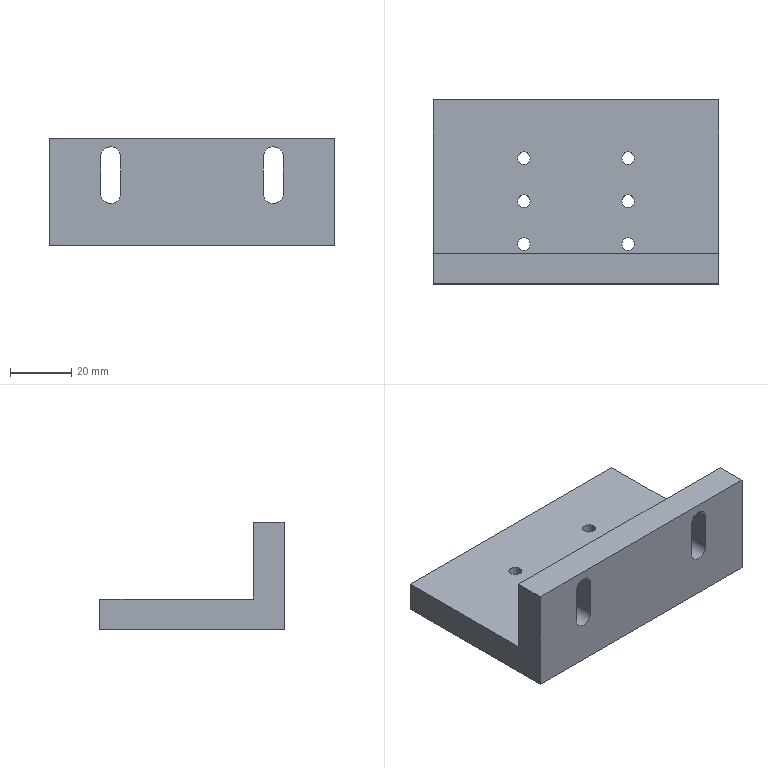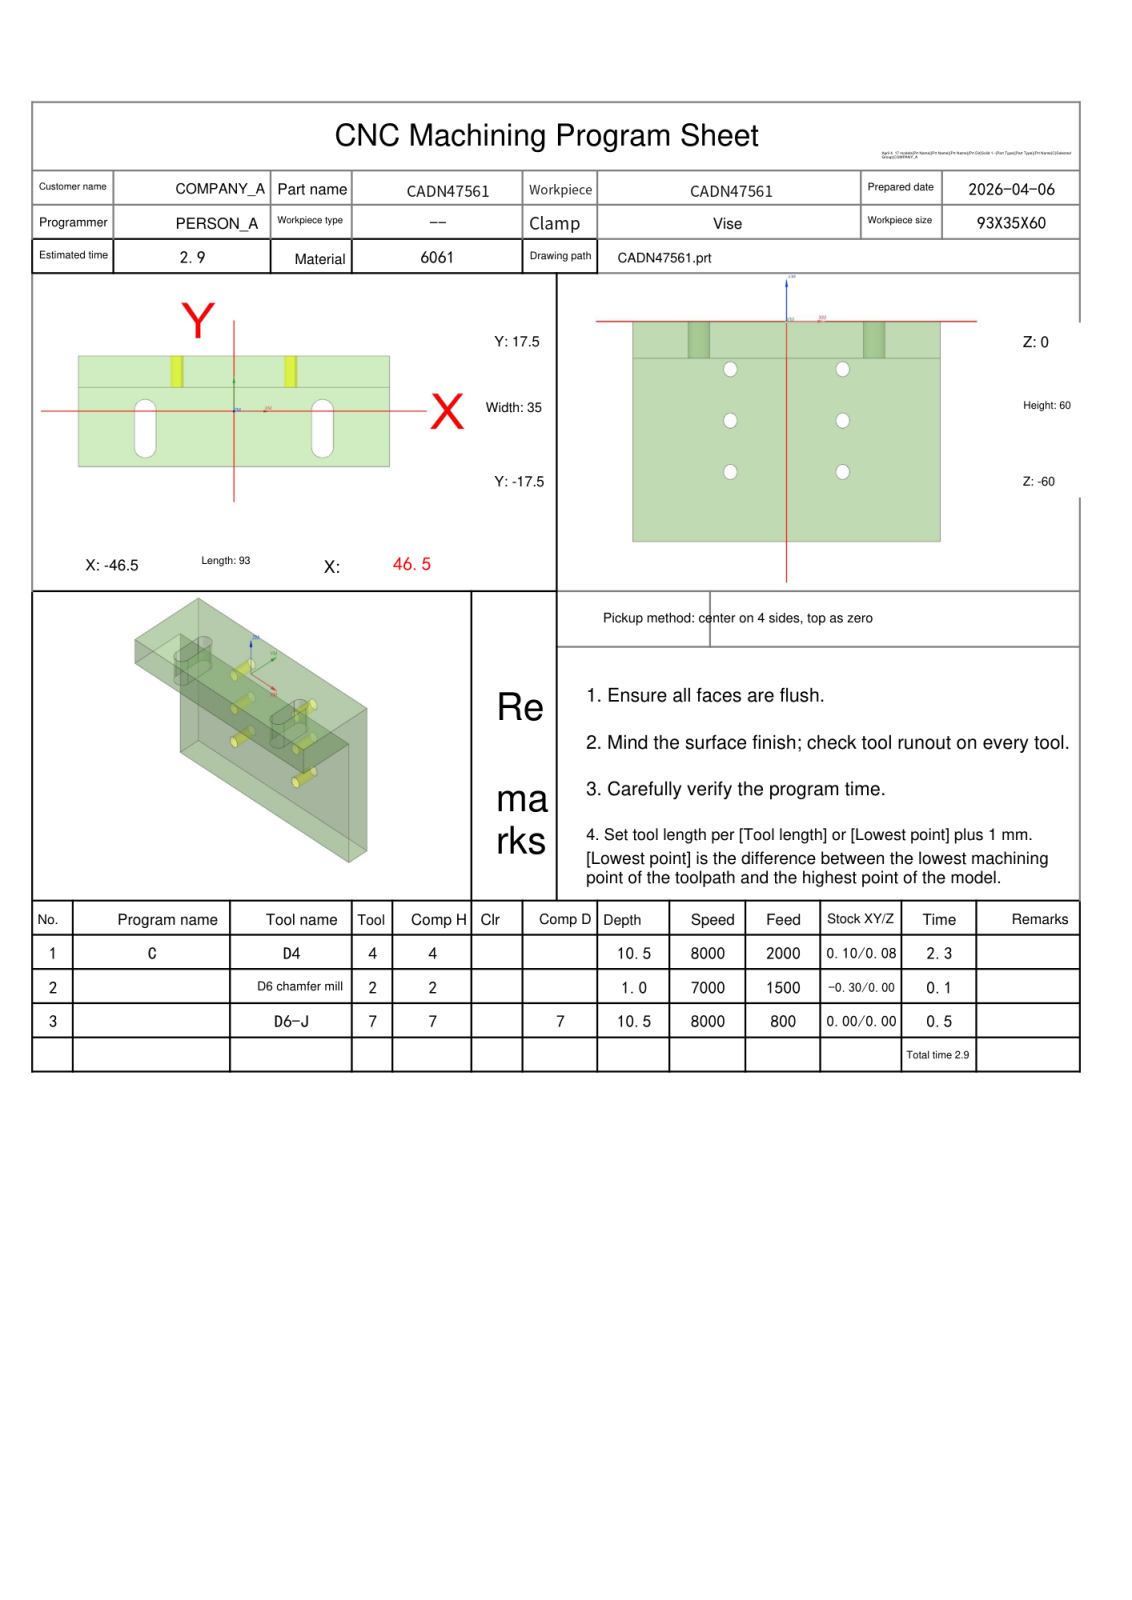NC program | NX | posted by the shop | part box 93 x 60 x 35 mm
Whole program:
%
O0001
(Machine time: 3.44 MIN)
(===Total Tool:3===)
(T4=D4      D=4.   R=0.   D-  H04 Z=-10.5 )
(T2=D6 chamfer mill   D=6.   R=0.   D-  H02 Z=-1.   )
(T7=D6-J    D=6.   R=0.   D7  H07 Z=-10.5 )
G80 G90 G17 G49 G40
G91 G28 Z0
M01
N1 T04 M06
(D4  D=4. R=0. H=04 ce=0.10 di=0.08)
G00 G90 G54 X-27.65 Y.101 M03 S8000
G43 H04 Z50.
M08
Z.8
G01 Y-11.5 Z.192 F2000.
Y-11.764 Z.178
X-27.334 Y-12.334 Z.144
X-26.764 Y-12.65 Z.11
X-26.236 Z.082
X-25.666 Y-12.334 Z.048
X-25.35 Y-11.764 Z.014
Y-11.5 Z0.0
Y.5 Z-.058
G03 X-26.5 Y1.65 Z-.066 I-1.15 J0.0
X-27.65 Y.5 Z-.075 I0.0 J-1.15
G01 Y-11.5 Z-.133
G03 X-26.5 Y-12.65 Z-.141 I1.15 J0.0
X-25.35 Y-11.5 Z-.15 I0.0 J1.15
G01 Y.5 Z-.208
G03 X-26.5 Y1.65 Z-.216 I-1.15 J0.0
X-27.65 Y.5 Z-.225 I0.0 J-1.15
G01 Y-11.5 Z-.283
G03 X-26.5 Y-12.65 Z-.291 I1.15 J0.0
X-25.35 Y-11.5 Z-.3 I0.0 J1.15
G01 Y.5 Z-.358
G03 X-26.5 Y1.65 Z-.366 I-1.15 J0.0
X-27.65 Y.5 Z-.375 I0.0 J-1.15
G01 Y-11.5 Z-.433
G03 X-26.5 Y-12.65 Z-.441 I1.15 J0.0
X-25.35 Y-11.5 Z-.45 I0.0 J1.15
G01 Y.5 Z-.508
G03 X-26.5 Y1.65 Z-.516 I-1.15 J0.0
X-27.65 Y.5 Z-.525 I0.0 J-1.15
G01 Y-11.5 Z-.583
G03 X-26.5 Y-12.65 Z-.591 I1.15 J0.0
X-25.35 Y-11.5 Z-.6 I0.0 J1.15
G01 Y.5 Z-.658
G03 X-26.5 Y1.65 Z-.666 I-1.15 J0.0
X-27.65 Y.5 Z-.675 I0.0 J-1.15
G01 Y-11.5 Z-.733
G03 X-26.5 Y-12.65 Z-.741 I1.15 J0.0
X-25.35 Y-11.5 Z-.75 I0.0 J1.15
G01 Y.5 Z-.808
G03 X-26.5 Y1.65 Z-.816 I-1.15 J0.0
X-27.65 Y.5 Z-.825 I0.0 J-1.15
G01 Y-11.5 Z-.883
G03 X-26.5 Y-12.65 Z-.891 I1.15 J0.0
X-25.35 Y-11.5 Z-.9 I0.0 J1.15
G01 Y.5 Z-.958
G03 X-26.5 Y1.65 Z-.966 I-1.15 J0.0
X-27.65 Y.5 Z-.975 I0.0 J-1.15
G01 Y-11.5 Z-1.033
G03 X-26.5 Y-12.65 Z-1.041 I1.15 J0.0
X-25.35 Y-11.5 Z-1.05 I0.0 J1.15
G01 Y.5 Z-1.108
G03 X-26.5 Y1.65 Z-1.116 I-1.15 J0.0
X-27.65 Y.5 Z-1.125 I0.0 J-1.15
G01 Y-11.5 Z-1.183
G03 X-26.5 Y-12.65 Z-1.191 I1.15 J0.0
X-25.35 Y-11.5 Z-1.2 I0.0 J1.15
G01 Y.5 Z-1.258
G03 X-26.5 Y1.65 Z-1.266 I-1.15 J0.0
X-27.65 Y.5 Z-1.275 I0.0 J-1.15
G01 Y-11.5 Z-1.333
G03 X-26.5 Y-12.65 Z-1.341 I1.15 J0.0
X-25.35 Y-11.5 Z-1.35 I0.0 J1.15
G01 Y.5 Z-1.408
G03 X-26.5 Y1.65 Z-1.416 I-1.15 J0.0
X-27.65 Y.5 Z-1.425 I0.0 J-1.15
G01 Y-11.5 Z-1.483
G03 X-26.5 Y-12.65 Z-1.491 I1.15 J0.0
X-25.35 Y-11.5 Z-1.5 I0.0 J1.15
G01 Y.5 Z-1.558
G03 X-26.5 Y1.65 Z-1.566 I-1.15 J0.0
X-27.65 Y.5 Z-1.575 I0.0 J-1.15
G01 Y-11.5 Z-1.633
G03 X-26.5 Y-12.65 Z-1.641 I1.15 J0.0
X-25.35 Y-11.5 Z-1.65 I0.0 J1.15
G01 Y.5 Z-1.708
G03 X-26.5 Y1.65 Z-1.716 I-1.15 J0.0
X-27.65 Y.5 Z-1.725 I0.0 J-1.15
G01 Y-11.5 Z-1.783
G03 X-26.5 Y-12.65 Z-1.791 I1.15 J0.0
X-25.35 Y-11.5 Z-1.8 I0.0 J1.15
G01 Y.5 Z-1.858
G03 X-26.5 Y1.65 Z-1.866 I-1.15 J0.0
X-27.65 Y.5 Z-1.875 I0.0 J-1.15
G01 Y-11.5 Z-1.933
G03 X-26.5 Y-12.65 Z-1.941 I1.15 J0.0
X-25.35 Y-11.5 Z-1.95 I0.0 J1.15
G01 Y.5 Z-2.008
G03 X-26.5 Y1.65 Z-2.016 I-1.15 J0.0
X-27.65 Y.5 Z-2.025 I0.0 J-1.15
G01 Y-11.5 Z-2.083
G03 X-26.5 Y-12.65 Z-2.091 I1.15 J0.0
X-25.35 Y-11.5 Z-2.1 I0.0 J1.15
G01 Y.5 Z-2.158
G03 X-26.5 Y1.65 Z-2.166 I-1.15 J0.0
X-27.65 Y.5 Z-2.175 I0.0 J-1.15
G01 Y-11.5 Z-2.233
G03 X-26.5 Y-12.65 Z-2.241 I1.15 J0.0
X-25.35 Y-11.5 Z-2.25 I0.0 J1.15
G01 Y.5 Z-2.308
G03 X-26.5 Y1.65 Z-2.316 I-1.15 J0.0
X-27.65 Y.5 Z-2.325 I0.0 J-1.15
G01 Y-11.5 Z-2.383
G03 X-26.5 Y-12.65 Z-2.391 I1.15 J0.0
X-25.35 Y-11.5 Z-2.4 I0.0 J1.15
G01 Y.5 Z-2.458
G03 X-26.5 Y1.65 Z-2.466 I-1.15 J0.0
X-27.65 Y.5 Z-2.475 I0.0 J-1.15
G01 Y-11.5 Z-2.533
G03 X-26.5 Y-12.65 Z-2.541 I1.15 J0.0
X-25.35 Y-11.5 Z-2.55 I0.0 J1.15
G01 Y.5 Z-2.608
G03 X-26.5 Y1.65 Z-2.616 I-1.15 J0.0
X-27.65 Y.5 Z-2.625 I0.0 J-1.15
G01 Y-11.5 Z-2.683
G03 X-26.5 Y-12.65 Z-2.691 I1.15 J0.0
X-25.35 Y-11.5 Z-2.7 I0.0 J1.15
G01 Y.5 Z-2.758
G03 X-26.5 Y1.65 Z-2.766 I-1.15 J0.0
X-27.65 Y.5 Z-2.775 I0.0 J-1.15
G01 Y-11.5 Z-2.833
G03 X-26.5 Y-12.65 Z-2.841 I1.15 J0.0
X-25.35 Y-11.5 Z-2.85 I0.0 J1.15
G01 Y.5 Z-2.908
G03 X-26.5 Y1.65 Z-2.916 I-1.15 J0.0
X-27.65 Y.5 Z-2.925 I0.0 J-1.15
G01 Y-11.5 Z-2.983
G03 X-26.5 Y-12.65 Z-2.991 I1.15 J0.0
X-25.35 Y-11.5 Z-3. I0.0 J1.15
G01 Y.5 Z-3.058
G03 X-26.5 Y1.65 Z-3.066 I-1.15 J0.0
X-27.65 Y.5 Z-3.075 I0.0 J-1.15
G01 Y-11.5 Z-3.133
G03 X-26.5 Y-12.65 Z-3.141 I1.15 J0.0
X-25.35 Y-11.5 Z-3.15 I0.0 J1.15
G01 Y.5 Z-3.208
G03 X-26.5 Y1.65 Z-3.216 I-1.15 J0.0
X-27.65 Y.5 Z-3.225 I0.0 J-1.15
G01 Y-11.5 Z-3.283
G03 X-26.5 Y-12.65 Z-3.291 I1.15 J0.0
X-25.35 Y-11.5 Z-3.3 I0.0 J1.15
G01 Y.5 Z-3.358
G03 X-26.5 Y1.65 Z-3.366 I-1.15 J0.0
X-27.65 Y.5 Z-3.375 I0.0 J-1.15
G01 Y-11.5 Z-3.433
G03 X-26.5 Y-12.65 Z-3.441 I1.15 J0.0
X-25.35 Y-11.5 Z-3.45 I0.0 J1.15
G01 Y.5 Z-3.508
G03 X-26.5 Y1.65 Z-3.516 I-1.15 J0.0
X-27.65 Y.5 Z-3.525 I0.0 J-1.15
G01 Y-11.5 Z-3.583
G03 X-26.5 Y-12.65 Z-3.591 I1.15 J0.0
X-25.35 Y-11.5 Z-3.6 I0.0 J1.15
G01 Y.5 Z-3.658
G03 X-26.5 Y1.65 Z-3.666 I-1.15 J0.0
X-27.65 Y.5 Z-3.675 I0.0 J-1.15
G01 Y-11.5 Z-3.733
G03 X-26.5 Y-12.65 Z-3.741 I1.15 J0.0
X-25.35 Y-11.5 Z-3.75 I0.0 J1.15
G01 Y.5 Z-3.808
G03 X-26.5 Y1.65 Z-3.816 I-1.15 J0.0
X-27.65 Y.5 Z-3.825 I0.0 J-1.15
G01 Y-11.5 Z-3.883
G03 X-26.5 Y-12.65 Z-3.891 I1.15 J0.0
X-25.35 Y-11.5 Z-3.9 I0.0 J1.15
G01 Y.5 Z-3.958
G03 X-26.5 Y1.65 Z-3.966 I-1.15 J0.0
X-27.65 Y.5 Z-3.975 I0.0 J-1.15
G01 Y-11.5 Z-4.033
G03 X-26.5 Y-12.65 Z-4.041 I1.15 J0.0
X-25.35 Y-11.5 Z-4.05 I0.0 J1.15
G01 Y.5 Z-4.108
G03 X-26.5 Y1.65 Z-4.116 I-1.15 J0.0
X-27.65 Y.5 Z-4.125 I0.0 J-1.15
G01 Y-11.5 Z-4.183
G03 X-26.5 Y-12.65 Z-4.191 I1.15 J0.0
X-25.35 Y-11.5 Z-4.2 I0.0 J1.15
G01 Y.5 Z-4.258
G03 X-26.5 Y1.65 Z-4.266 I-1.15 J0.0
X-27.65 Y.5 Z-4.275 I0.0 J-1.15
G01 Y-11.5 Z-4.333
G03 X-26.5 Y-12.65 Z-4.341 I1.15 J0.0
X-25.35 Y-11.5 Z-4.35 I0.0 J1.15
G01 Y.5 Z-4.408
G03 X-26.5 Y1.65 Z-4.416 I-1.15 J0.0
X-27.65 Y.5 Z-4.425 I0.0 J-1.15
G01 Y-11.5 Z-4.483
G03 X-26.5 Y-12.65 Z-4.491 I1.15 J0.0
X-25.35 Y-11.5 Z-4.5 I0.0 J1.15
G01 Y.5 Z-4.558
G03 X-26.5 Y1.65 Z-4.566 I-1.15 J0.0
X-27.65 Y.5 Z-4.575 I0.0 J-1.15
G01 Y-11.5 Z-4.633
G03 X-26.5 Y-12.65 Z-4.641 I1.15 J0.0
X-25.35 Y-11.5 Z-4.65 I0.0 J1.15
G01 Y.5 Z-4.708
G03 X-26.5 Y1.65 Z-4.716 I-1.15 J0.0
X-27.65 Y.5 Z-4.725 I0.0 J-1.15
G01 Y-11.5 Z-4.783
G03 X-26.5 Y-12.65 Z-4.791 I1.15 J0.0
X-25.35 Y-11.5 Z-4.8 I0.0 J1.15
G01 Y.5 Z-4.858
G03 X-26.5 Y1.65 Z-4.866 I-1.15 J0.0
X-27.65 Y.5 Z-4.875 I0.0 J-1.15
G01 Y-11.5 Z-4.933
G03 X-26.5 Y-12.65 Z-4.941 I1.15 J0.0
X-25.35 Y-11.5 Z-4.95 I0.0 J1.15
G01 Y.5 Z-5.008
G03 X-26.5 Y1.65 Z-5.016 I-1.15 J0.0
X-27.65 Y.5 Z-5.025 I0.0 J-1.15
G01 Y-11.5 Z-5.083
G03 X-26.5 Y-12.65 Z-5.091 I1.15 J0.0
X-25.35 Y-11.5 Z-5.1 I0.0 J1.15
G01 Y.5 Z-5.158
G03 X-26.5 Y1.65 Z-5.166 I-1.15 J0.0
X-27.65 Y.5 Z-5.175 I0.0 J-1.15
G01 Y-11.5 Z-5.233
G03 X-26.5 Y-12.65 Z-5.241 I1.15 J0.0
X-25.35 Y-11.5 Z-5.25 I0.0 J1.15
G01 Y.5 Z-5.308
G03 X-26.5 Y1.65 Z-5.316 I-1.15 J0.0
X-27.65 Y.5 Z-5.325 I0.0 J-1.15
G01 Y-11.5 Z-5.383
G03 X-26.5 Y-12.65 Z-5.391 I1.15 J0.0
X-25.35 Y-11.5 Z-5.4 I0.0 J1.15
G01 Y.5 Z-5.458
G03 X-26.5 Y1.65 Z-5.466 I-1.15 J0.0
X-27.65 Y.5 Z-5.475 I0.0 J-1.15
G01 Y-11.5 Z-5.533
G03 X-26.5 Y-12.65 Z-5.541 I1.15 J0.0
X-25.35 Y-11.5 Z-5.55 I0.0 J1.15
G01 Y.5 Z-5.608
G03 X-26.5 Y1.65 Z-5.616 I-1.15 J0.0
X-27.65 Y.5 Z-5.625 I0.0 J-1.15
G01 Y-11.5 Z-5.683
G03 X-26.5 Y-12.65 Z-5.691 I1.15 J0.0
X-25.35 Y-11.5 Z-5.7 I0.0 J1.15
G01 Y.5 Z-5.758
G03 X-26.5 Y1.65 Z-5.766 I-1.15 J0.0
X-27.65 Y.5 Z-5.775 I0.0 J-1.15
G01 Y-11.5 Z-5.833
G03 X-26.5 Y-12.65 Z-5.841 I1.15 J0.0
X-25.35 Y-11.5 Z-5.85 I0.0 J1.15
G01 Y.5 Z-5.908
G03 X-26.5 Y1.65 Z-5.916 I-1.15 J0.0
X-27.65 Y.5 Z-5.925 I0.0 J-1.15
G01 Y-11.5 Z-5.983
G03 X-26.5 Y-12.65 Z-5.991 I1.15 J0.0
X-25.35 Y-11.5 Z-6. I0.0 J1.15
G01 Y.5 Z-6.058
G03 X-26.5 Y1.65 Z-6.066 I-1.15 J0.0
X-27.65 Y.5 Z-6.075 I0.0 J-1.15
G01 Y-11.5 Z-6.133
G03 X-26.5 Y-12.65 Z-6.141 I1.15 J0.0
X-25.35 Y-11.5 Z-6.15 I0.0 J1.15
G01 Y.5 Z-6.208
G03 X-26.5 Y1.65 Z-6.216 I-1.15 J0.0
X-27.65 Y.5 Z-6.225 I0.0 J-1.15
G01 Y-11.5 Z-6.283
G03 X-26.5 Y-12.65 Z-6.291 I1.15 J0.0
X-25.35 Y-11.5 Z-6.3 I0.0 J1.15
G01 Y.5 Z-6.358
G03 X-26.5 Y1.65 Z-6.366 I-1.15 J0.0
X-27.65 Y.5 Z-6.375 I0.0 J-1.15
G01 Y-11.5 Z-6.433
G03 X-26.5 Y-12.65 Z-6.441 I1.15 J0.0
X-25.35 Y-11.5 Z-6.45 I0.0 J1.15
G01 Y.5 Z-6.508
G03 X-26.5 Y1.65 Z-6.516 I-1.15 J0.0
X-27.65 Y.5 Z-6.525 I0.0 J-1.15
G01 Y-11.5 Z-6.583
G03 X-26.5 Y-12.65 Z-6.591 I1.15 J0.0
X-25.35 Y-11.5 Z-6.6 I0.0 J1.15
G01 Y.5 Z-6.658
G03 X-26.5 Y1.65 Z-6.666 I-1.15 J0.0
X-27.65 Y.5 Z-6.675 I0.0 J-1.15
G01 Y-11.5 Z-6.733
G03 X-26.5 Y-12.65 Z-6.741 I1.15 J0.0
X-25.35 Y-11.5 Z-6.75 I0.0 J1.15
G01 Y.5 Z-6.808
G03 X-26.5 Y1.65 Z-6.816 I-1.15 J0.0
X-27.65 Y.5 Z-6.825 I0.0 J-1.15
G01 Y-11.5 Z-6.883
G03 X-26.5 Y-12.65 Z-6.891 I1.15 J0.0
X-25.35 Y-11.5 Z-6.9 I0.0 J1.15
G01 Y.5 Z-6.958
G03 X-26.5 Y1.65 Z-6.966 I-1.15 J0.0
X-27.65 Y.5 Z-6.975 I0.0 J-1.15
G01 Y-11.5 Z-7.033
G03 X-26.5 Y-12.65 Z-7.041 I1.15 J0.0
X-25.35 Y-11.5 Z-7.05 I0.0 J1.15
G01 Y.5 Z-7.108
G03 X-26.5 Y1.65 Z-7.116 I-1.15 J0.0
X-27.65 Y.5 Z-7.125 I0.0 J-1.15
G01 Y-11.5 Z-7.183
G03 X-26.5 Y-12.65 Z-7.191 I1.15 J0.0
X-25.35 Y-11.5 Z-7.2 I0.0 J1.15
G01 Y.5 Z-7.258
G03 X-26.5 Y1.65 Z-7.266 I-1.15 J0.0
X-27.65 Y.5 Z-7.275 I0.0 J-1.15
G01 Y-11.5 Z-7.333
G03 X-26.5 Y-12.65 Z-7.341 I1.15 J0.0
X-25.35 Y-11.5 Z-7.35 I0.0 J1.15
G01 Y.5 Z-7.408
G03 X-26.5 Y1.65 Z-7.416 I-1.15 J0.0
X-27.65 Y.5 Z-7.425 I0.0 J-1.15
G01 Y-11.5 Z-7.483
G03 X-26.5 Y-12.65 Z-7.491 I1.15 J0.0
X-25.35 Y-11.5 Z-7.5 I0.0 J1.15
G01 Y.5 Z-7.558
G03 X-26.5 Y1.65 Z-7.566 I-1.15 J0.0
X-27.65 Y.5 Z-7.575 I0.0 J-1.15
G01 Y-11.5 Z-7.633
G03 X-26.5 Y-12.65 Z-7.641 I1.15 J0.0
X-25.35 Y-11.5 Z-7.65 I0.0 J1.15
G01 Y.5 Z-7.708
G03 X-26.5 Y1.65 Z-7.716 I-1.15 J0.0
X-27.65 Y.5 Z-7.725 I0.0 J-1.15
G01 Y-11.5 Z-7.783
G03 X-26.5 Y-12.65 Z-7.791 I1.15 J0.0
X-25.35 Y-11.5 Z-7.8 I0.0 J1.15
G01 Y.5 Z-7.858
G03 X-26.5 Y1.65 Z-7.866 I-1.15 J0.0
X-27.65 Y.5 Z-7.875 I0.0 J-1.15
G01 Y-11.5 Z-7.933
G03 X-26.5 Y-12.65 Z-7.941 I1.15 J0.0
X-25.35 Y-11.5 Z-7.95 I0.0 J1.15
G01 Y.5 Z-8.008
G03 X-26.5 Y1.65 Z-8.016 I-1.15 J0.0
X-27.65 Y.5 Z-8.025 I0.0 J-1.15
G01 Y-11.5 Z-8.083
G03 X-26.5 Y-12.65 Z-8.091 I1.15 J0.0
X-25.35 Y-11.5 Z-8.1 I0.0 J1.15
G01 Y.5 Z-8.158
G03 X-26.5 Y1.65 Z-8.166 I-1.15 J0.0
X-27.65 Y.5 Z-8.175 I0.0 J-1.15
G01 Y-11.5 Z-8.233
G03 X-26.5 Y-12.65 Z-8.241 I1.15 J0.0
X-25.35 Y-11.5 Z-8.25 I0.0 J1.15
G01 Y.5 Z-8.308
G03 X-26.5 Y1.65 Z-8.316 I-1.15 J0.0
X-27.65 Y.5 Z-8.325 I0.0 J-1.15
G01 Y-11.5 Z-8.383
G03 X-26.5 Y-12.65 Z-8.391 I1.15 J0.0
X-25.35 Y-11.5 Z-8.4 I0.0 J1.15
G01 Y.5 Z-8.458
G03 X-26.5 Y1.65 Z-8.466 I-1.15 J0.0
X-27.65 Y.5 Z-8.475 I0.0 J-1.15
G01 Y-11.5 Z-8.533
G03 X-26.5 Y-12.65 Z-8.541 I1.15 J0.0
X-25.35 Y-11.5 Z-8.55 I0.0 J1.15
G01 Y.5 Z-8.608
G03 X-26.5 Y1.65 Z-8.616 I-1.15 J0.0
X-27.65 Y.5 Z-8.625 I0.0 J-1.15
G01 Y-11.5 Z-8.683
G03 X-26.5 Y-12.65 Z-8.691 I1.15 J0.0
X-25.35 Y-11.5 Z-8.7 I0.0 J1.15
G01 Y.5 Z-8.758
G03 X-26.5 Y1.65 Z-8.766 I-1.15 J0.0
X-27.65 Y.5 Z-8.775 I0.0 J-1.15
G01 Y-11.5 Z-8.833
G03 X-26.5 Y-12.65 Z-8.841 I1.15 J0.0
X-25.35 Y-11.5 Z-8.85 I0.0 J1.15
G01 Y.5 Z-8.908
G03 X-26.5 Y1.65 Z-8.916 I-1.15 J0.0
X-27.65 Y.5 Z-8.925 I0.0 J-1.15
G01 Y-11.5 Z-8.983
G03 X-26.5 Y-12.65 Z-8.991 I1.15 J0.0
X-25.35 Y-11.5 Z-9. I0.0 J1.15
G01 Y.5 Z-9.058
G03 X-26.5 Y1.65 Z-9.066 I-1.15 J0.0
X-27.65 Y.5 Z-9.075 I0.0 J-1.15
G01 Y-11.5 Z-9.133
G03 X-26.5 Y-12.65 Z-9.141 I1.15 J0.0
X-25.35 Y-11.5 Z-9.15 I0.0 J1.15
G01 Y.5 Z-9.208
G03 X-26.5 Y1.65 Z-9.216 I-1.15 J0.0
X-27.65 Y.5 Z-9.225 I0.0 J-1.15
G01 Y-11.5 Z-9.283
G03 X-26.5 Y-12.65 Z-9.291 I1.15 J0.0
X-25.35 Y-11.5 Z-9.3 I0.0 J1.15
G01 Y.5 Z-9.358
G03 X-26.5 Y1.65 Z-9.366 I-1.15 J0.0
X-27.65 Y.5 Z-9.375 I0.0 J-1.15
G01 Y-11.5 Z-9.433
G03 X-26.5 Y-12.65 Z-9.441 I1.15 J0.0
X-25.35 Y-11.5 Z-9.45 I0.0 J1.15
G01 Y.5 Z-9.508
G03 X-26.5 Y1.65 Z-9.516 I-1.15 J0.0
X-27.65 Y.5 Z-9.525 I0.0 J-1.15
G01 Y-11.5 Z-9.583
G03 X-26.5 Y-12.65 Z-9.591 I1.15 J0.0
X-25.35 Y-11.5 Z-9.6 I0.0 J1.15
G01 Y.5 Z-9.658
G03 X-26.5 Y1.65 Z-9.666 I-1.15 J0.0
X-27.65 Y.5 Z-9.675 I0.0 J-1.15
G01 Y-11.5 Z-9.733
G03 X-26.5 Y-12.65 Z-9.741 I1.15 J0.0
X-25.35 Y-11.5 Z-9.75 I0.0 J1.15
G01 Y.5 Z-9.808
G03 X-26.5 Y1.65 Z-9.816 I-1.15 J0.0
X-27.65 Y.5 Z-9.825 I0.0 J-1.15
G01 Y-11.5 Z-9.883
G03 X-26.5 Y-12.65 Z-9.891 I1.15 J0.0
X-25.35 Y-11.5 Z-9.9 I0.0 J1.15
G01 Y.5 Z-9.958
G03 X-26.5 Y1.65 Z-9.966 I-1.15 J0.0
X-27.65 Y.5 Z-9.975 I0.0 J-1.15
G01 Y-11.5 Z-10.033
G03 X-26.5 Y-12.65 Z-10.041 I1.15 J0.0
X-25.35 Y-11.5 Z-10.05 I0.0 J1.15
G01 Y.5 Z-10.108
G03 X-26.5 Y1.65 Z-10.116 I-1.15 J0.0
X-27.65 Y.5 Z-10.125 I0.0 J-1.15
G01 Y-11.5 Z-10.183
G03 X-26.5 Y-12.65 Z-10.191 I1.15 J0.0
X-25.35 Y-11.5 Z-10.2 I0.0 J1.15
G01 Y.5 Z-10.258
G03 X-26.5 Y1.65 Z-10.266 I-1.15 J0.0
X-27.65 Y.5 Z-10.275 I0.0 J-1.15
G01 Y-11.5 Z-10.333
G03 X-26.5 Y-12.65 Z-10.341 I1.15 J0.0
X-25.35 Y-11.5 Z-10.35 I0.0 J1.15
G01 Y.5 Z-10.408
G03 X-26.5 Y1.65 Z-10.416 I-1.15 J0.0
X-27.65 Y.5 Z-10.425 I0.0 J-1.15
G01 Y-11.5 Z-10.483
G03 X-26.5 Y-12.65 Z-10.491 I1.15 J0.0
X-25.35 Y-11.5 Z-10.5 I0.0 J1.15
G01 Y.5
G03 X-26.5 Y1.65 I-1.15 J0.0
X-27.65 Y.5 I0.0 J-1.15
G01 Y-11.5
G03 X-26.5 Y-12.65 I1.15 J0.0
X-25.35 Y-11.5 I0.0 J1.15
G01 Y-11.1
Z-9.7
G00 Z50.
X27.65 Y-11.101
Z.8
G01 Y.764 Z.178
X27.334 Y1.334 Z.144
X26.764 Y1.65 Z.11
X26.236 Z.082
X25.666 Y1.334 Z.048
X25.35 Y.764 Z.014
Y.5 Z0.0
Y-11.5 Z-.058
G03 X26.5 Y-12.65 Z-.066 I1.15 J0.0
X27.65 Y-11.5 Z-.075 I0.0 J1.15
G01 Y.5 Z-.133
G03 X26.5 Y1.65 Z-.141 I-1.15 J0.0
X25.35 Y.5 Z-.15 I0.0 J-1.15
G01 Y-11.5 Z-.208
G03 X26.5 Y-12.65 Z-.216 I1.15 J0.0
X27.65 Y-11.5 Z-.225 I0.0 J1.15
G01 Y.5 Z-.283
G03 X26.5 Y1.65 Z-.291 I-1.15 J0.0
X25.35 Y.5 Z-.3 I0.0 J-1.15
G01 Y-11.5 Z-.358
G03 X26.5 Y-12.65 Z-.366 I1.15 J0.0
X27.65 Y-11.5 Z-.375 I0.0 J1.15
G01 Y.5 Z-.433
G03 X26.5 Y1.65 Z-.441 I-1.15 J0.0
X25.35 Y.5 Z-.45 I0.0 J-1.15
G01 Y-11.5 Z-.508
G03 X26.5 Y-12.65 Z-.516 I1.15 J0.0
X27.65 Y-11.5 Z-.525 I0.0 J1.15
G01 Y.5 Z-.583
G03 X26.5 Y1.65 Z-.591 I-1.15 J0.0
X25.35 Y.5 Z-.6 I0.0 J-1.15
G01 Y-11.5 Z-.658
G03 X26.5 Y-12.65 Z-.666 I1.15 J0.0
X27.65 Y-11.5 Z-.675 I0.0 J1.15
G01 Y.5 Z-.733
G03 X26.5 Y1.65 Z-.741 I-1.15 J0.0
X25.35 Y.5 Z-.75 I0.0 J-1.15
G01 Y-11.5 Z-.808
G03 X26.5 Y-12.65 Z-.816 I1.15 J0.0
X27.65 Y-11.5 Z-.825 I0.0 J1.15
G01 Y.5 Z-.883
G03 X26.5 Y1.65 Z-.891 I-1.15 J0.0
X25.35 Y.5 Z-.9 I0.0 J-1.15
G01 Y-11.5 Z-.958
G03 X26.5 Y-12.65 Z-.966 I1.15 J0.0
X27.65 Y-11.5 Z-.975 I0.0 J1.15
G01 Y.5 Z-1.033
G03 X26.5 Y1.65 Z-1.041 I-1.15 J0.0
X25.35 Y.5 Z-1.05 I0.0 J-1.15
G01 Y-11.5 Z-1.108
G03 X26.5 Y-12.65 Z-1.116 I1.15 J0.0
X27.65 Y-11.5 Z-1.125 I0.0 J1.15
G01 Y.5 Z-1.183
G03 X26.5 Y1.65 Z-1.191 I-1.15 J0.0
X25.35 Y.5 Z-1.2 I0.0 J-1.15
G01 Y-11.5 Z-1.258
G03 X26.5 Y-12.65 Z-1.266 I1.15 J0.0
X27.65 Y-11.5 Z-1.275 I0.0 J1.15
G01 Y.5 Z-1.333
G03 X26.5 Y1.65 Z-1.341 I-1.15 J0.0
X25.35 Y.5 Z-1.35 I0.0 J-1.15
G01 Y-11.5 Z-1.408
G03 X26.5 Y-12.65 Z-1.416 I1.15 J0.0
X27.65 Y-11.5 Z-1.425 I0.0 J1.15
G01 Y.5 Z-1.483
G03 X26.5 Y1.65 Z-1.491 I-1.15 J0.0
X25.35 Y.5 Z-1.5 I0.0 J-1.15
G01 Y-11.5 Z-1.558
G03 X26.5 Y-12.65 Z-1.566 I1.15 J0.0
X27.65 Y-11.5 Z-1.575 I0.0 J1.15
G01 Y.5 Z-1.633
G03 X26.5 Y1.65 Z-1.641 I-1.15 J0.0
X25.35 Y.5 Z-1.65 I0.0 J-1.15
G01 Y-11.5 Z-1.708
G03 X26.5 Y-12.65 Z-1.716 I1.15 J0.0
X27.65 Y-11.5 Z-1.725 I0.0 J1.15
G01 Y.5 Z-1.783
G03 X26.5 Y1.65 Z-1.791 I-1.15 J0.0
X25.35 Y.5 Z-1.8 I0.0 J-1.15
G01 Y-11.5 Z-1.858
G03 X26.5 Y-12.65 Z-1.866 I1.15 J0.0
X27.65 Y-11.5 Z-1.875 I0.0 J1.15
G01 Y.5 Z-1.933
G03 X26.5 Y1.65 Z-1.941 I-1.15 J0.0
X25.35 Y.5 Z-1.95 I0.0 J-1.15
G01 Y-11.5 Z-2.008
G03 X26.5 Y-12.65 Z-2.016 I1.15 J0.0
X27.65 Y-11.5 Z-2.025 I0.0 J1.15
G01 Y.5 Z-2.083
G03 X26.5 Y1.65 Z-2.091 I-1.15 J0.0
X25.35 Y.5 Z-2.1 I0.0 J-1.15
G01 Y-11.5 Z-2.158
G03 X26.5 Y-12.65 Z-2.166 I1.15 J0.0
X27.65 Y-11.5 Z-2.175 I0.0 J1.15
G01 Y.5 Z-2.233
G03 X26.5 Y1.65 Z-2.241 I-1.15 J0.0
X25.35 Y.5 Z-2.25 I0.0 J-1.15
G01 Y-11.5 Z-2.308
G03 X26.5 Y-12.65 Z-2.316 I1.15 J0.0
X27.65 Y-11.5 Z-2.325 I0.0 J1.15
G01 Y.5 Z-2.383
G03 X26.5 Y1.65 Z-2.391 I-1.15 J0.0
X25.35 Y.5 Z-2.4 I0.0 J-1.15
G01 Y-11.5 Z-2.458
G03 X26.5 Y-12.65 Z-2.466 I1.15 J0.0
X27.65 Y-11.5 Z-2.475 I0.0 J1.15
G01 Y.5 Z-2.533
G03 X26.5 Y1.65 Z-2.541 I-1.15 J0.0
X25.35 Y.5 Z-2.55 I0.0 J-1.15
G01 Y-11.5 Z-2.608
G03 X26.5 Y-12.65 Z-2.616 I1.15 J0.0
X27.65 Y-11.5 Z-2.625 I0.0 J1.15
G01 Y.5 Z-2.683
G03 X26.5 Y1.65 Z-2.691 I-1.15 J0.0
X25.35 Y.5 Z-2.7 I0.0 J-1.15
G01 Y-11.5 Z-2.758
G03 X26.5 Y-12.65 Z-2.766 I1.15 J0.0
X27.65 Y-11.5 Z-2.775 I0.0 J1.15
G01 Y.5 Z-2.833
G03 X26.5 Y1.65 Z-2.841 I-1.15 J0.0
X25.35 Y.5 Z-2.85 I0.0 J-1.15
G01 Y-11.5 Z-2.908
G03 X26.5 Y-12.65 Z-2.916 I1.15 J0.0
X27.65 Y-11.5 Z-2.925 I0.0 J1.15
G01 Y.5 Z-2.983
G03 X26.5 Y1.65 Z-2.991 I-1.15 J0.0
X25.35 Y.5 Z-3. I0.0 J-1.15
G01 Y-11.5 Z-3.058
G03 X26.5 Y-12.65 Z-3.066 I1.15 J0.0
X27.65 Y-11.5 Z-3.075 I0.0 J1.15
G01 Y.5 Z-3.133
G03 X26.5 Y1.65 Z-3.141 I-1.15 J0.0
X25.35 Y.5 Z-3.15 I0.0 J-1.15
G01 Y-11.5 Z-3.208
G03 X26.5 Y-12.65 Z-3.216 I1.15 J0.0
X27.65 Y-11.5 Z-3.225 I0.0 J1.15
G01 Y.5 Z-3.283
G03 X26.5 Y1.65 Z-3.291 I-1.15 J0.0
X25.35 Y.5 Z-3.3 I0.0 J-1.15
G01 Y-11.5 Z-3.358
G03 X26.5 Y-12.65 Z-3.366 I1.15 J0.0
X27.65 Y-11.5 Z-3.375 I0.0 J1.15
G01 Y.5 Z-3.433
G03 X26.5 Y1.65 Z-3.441 I-1.15 J0.0
X25.35 Y.5 Z-3.45 I0.0 J-1.15
G01 Y-11.5 Z-3.508
G03 X26.5 Y-12.65 Z-3.516 I1.15 J0.0
X27.65 Y-11.5 Z-3.525 I0.0 J1.15
G01 Y.5 Z-3.583
G03 X26.5 Y1.65 Z-3.591 I-1.15 J0.0
X25.35 Y.5 Z-3.6 I0.0 J-1.15
G01 Y-11.5 Z-3.658
G03 X26.5 Y-12.65 Z-3.666 I1.15 J0.0
X27.65 Y-11.5 Z-3.675 I0.0 J1.15
G01 Y.5 Z-3.733
G03 X26.5 Y1.65 Z-3.741 I-1.15 J0.0
X25.35 Y.5 Z-3.75 I0.0 J-1.15
G01 Y-11.5 Z-3.808
G03 X26.5 Y-12.65 Z-3.816 I1.15 J0.0
X27.65 Y-11.5 Z-3.825 I0.0 J1.15
G01 Y.5 Z-3.883
G03 X26.5 Y1.65 Z-3.891 I-1.15 J0.0
X25.35 Y.5 Z-3.9 I0.0 J-1.15
G01 Y-11.5 Z-3.958
G03 X26.5 Y-12.65 Z-3.966 I1.15 J0.0
X27.65 Y-11.5 Z-3.975 I0.0 J1.15
G01 Y.5 Z-4.033
G03 X26.5 Y1.65 Z-4.041 I-1.15 J0.0
X25.35 Y.5 Z-4.05 I0.0 J-1.15
G01 Y-11.5 Z-4.108
G03 X26.5 Y-12.65 Z-4.116 I1.15 J0.0
X27.65 Y-11.5 Z-4.125 I0.0 J1.15
G01 Y.5 Z-4.183
G03 X26.5 Y1.65 Z-4.191 I-1.15 J0.0
X25.35 Y.5 Z-4.2 I0.0 J-1.15
G01 Y-11.5 Z-4.258
G03 X26.5 Y-12.65 Z-4.266 I1.15 J0.0
X27.65 Y-11.5 Z-4.275 I0.0 J1.15
G01 Y.5 Z-4.333
G03 X26.5 Y1.65 Z-4.341 I-1.15 J0.0
X25.35 Y.5 Z-4.35 I0.0 J-1.15
G01 Y-11.5 Z-4.408
G03 X26.5 Y-12.65 Z-4.416 I1.15 J0.0
X27.65 Y-11.5 Z-4.425 I0.0 J1.15
G01 Y.5 Z-4.483
G03 X26.5 Y1.65 Z-4.491 I-1.15 J0.0
X25.35 Y.5 Z-4.5 I0.0 J-1.15
G01 Y-11.5 Z-4.558
G03 X26.5 Y-12.65 Z-4.566 I1.15 J0.0
X27.65 Y-11.5 Z-4.575 I0.0 J1.15
G01 Y.5 Z-4.633
G03 X26.5 Y1.65 Z-4.641 I-1.15 J0.0
X25.35 Y.5 Z-4.65 I0.0 J-1.15
G01 Y-11.5 Z-4.708
G03 X26.5 Y-12.65 Z-4.716 I1.15 J0.0
X27.65 Y-11.5 Z-4.725 I0.0 J1.15
G01 Y.5 Z-4.783
G03 X26.5 Y1.65 Z-4.791 I-1.15 J0.0
X25.35 Y.5 Z-4.8 I0.0 J-1.15
G01 Y-11.5 Z-4.858
G03 X26.5 Y-12.65 Z-4.866 I1.15 J0.0
X27.65 Y-11.5 Z-4.875 I0.0 J1.15
G01 Y.5 Z-4.933
G03 X26.5 Y1.65 Z-4.941 I-1.15 J0.0
X25.35 Y.5 Z-4.95 I0.0 J-1.15
G01 Y-11.5 Z-5.008
G03 X26.5 Y-12.65 Z-5.016 I1.15 J0.0
X27.65 Y-11.5 Z-5.025 I0.0 J1.15
G01 Y.5 Z-5.083
G03 X26.5 Y1.65 Z-5.091 I-1.15 J0.0
X25.35 Y.5 Z-5.1 I0.0 J-1.15
G01 Y-11.5 Z-5.158
G03 X26.5 Y-12.65 Z-5.166 I1.15 J0.0
X27.65 Y-11.5 Z-5.175 I0.0 J1.15
G01 Y.5 Z-5.233
G03 X26.5 Y1.65 Z-5.241 I-1.15 J0.0
X25.35 Y.5 Z-5.25 I0.0 J-1.15
G01 Y-11.5 Z-5.308
G03 X26.5 Y-12.65 Z-5.316 I1.15 J0.0
X27.65 Y-11.5 Z-5.325 I0.0 J1.15
G01 Y.5 Z-5.383
G03 X26.5 Y1.65 Z-5.391 I-1.15 J0.0
X25.35 Y.5 Z-5.4 I0.0 J-1.15
G01 Y-11.5 Z-5.458
G03 X26.5 Y-12.65 Z-5.466 I1.15 J0.0
X27.65 Y-11.5 Z-5.475 I0.0 J1.15
G01 Y.5 Z-5.533
G03 X26.5 Y1.65 Z-5.541 I-1.15 J0.0
X25.35 Y.5 Z-5.55 I0.0 J-1.15
G01 Y-11.5 Z-5.608
G03 X26.5 Y-12.65 Z-5.616 I1.15 J0.0
X27.65 Y-11.5 Z-5.625 I0.0 J1.15
G01 Y.5 Z-5.683
G03 X26.5 Y1.65 Z-5.691 I-1.15 J0.0
X25.35 Y.5 Z-5.7 I0.0 J-1.15
G01 Y-11.5 Z-5.758
G03 X26.5 Y-12.65 Z-5.766 I1.15 J0.0
X27.65 Y-11.5 Z-5.775 I0.0 J1.15
G01 Y.5 Z-5.833
G03 X26.5 Y1.65 Z-5.841 I-1.15 J0.0
X25.35 Y.5 Z-5.85 I0.0 J-1.15
G01 Y-11.5 Z-5.908
G03 X26.5 Y-12.65 Z-5.916 I1.15 J0.0
X27.65 Y-11.5 Z-5.925 I0.0 J1.15
G01 Y.5 Z-5.983
G03 X26.5 Y1.65 Z-5.991 I-1.15 J0.0
X25.35 Y.5 Z-6. I0.0 J-1.15
G01 Y-11.5 Z-6.058
G03 X26.5 Y-12.65 Z-6.066 I1.15 J0.0
X27.65 Y-11.5 Z-6.075 I0.0 J1.15
G01 Y.5 Z-6.133
G03 X26.5 Y1.65 Z-6.141 I-1.15 J0.0
X25.35 Y.5 Z-6.15 I0.0 J-1.15
G01 Y-11.5 Z-6.208
G03 X26.5 Y-12.65 Z-6.216 I1.15 J0.0
X27.65 Y-11.5 Z-6.225 I0.0 J1.15
G01 Y.5 Z-6.283
G03 X26.5 Y1.65 Z-6.291 I-1.15 J0.0
X25.35 Y.5 Z-6.3 I0.0 J-1.15
G01 Y-11.5 Z-6.358
G03 X26.5 Y-12.65 Z-6.366 I1.15 J0.0
X27.65 Y-11.5 Z-6.375 I0.0 J1.15
G01 Y.5 Z-6.433
G03 X26.5 Y1.65 Z-6.441 I-1.15 J0.0
X25.35 Y.5 Z-6.45 I0.0 J-1.15
G01 Y-11.5 Z-6.508
G03 X26.5 Y-12.65 Z-6.516 I1.15 J0.0
X27.65 Y-11.5 Z-6.525 I0.0 J1.15
G01 Y.5 Z-6.583
G03 X26.5 Y1.65 Z-6.591 I-1.15 J0.0
X25.35 Y.5 Z-6.6 I0.0 J-1.15
G01 Y-11.5 Z-6.658
G03 X26.5 Y-12.65 Z-6.666 I1.15 J0.0
X27.65 Y-11.5 Z-6.675 I0.0 J1.15
G01 Y.5 Z-6.733
G03 X26.5 Y1.65 Z-6.741 I-1.15 J0.0
X25.35 Y.5 Z-6.75 I0.0 J-1.15
G01 Y-11.5 Z-6.808
G03 X26.5 Y-12.65 Z-6.816 I1.15 J0.0
X27.65 Y-11.5 Z-6.825 I0.0 J1.15
G01 Y.5 Z-6.883
G03 X26.5 Y1.65 Z-6.891 I-1.15 J0.0
X25.35 Y.5 Z-6.9 I0.0 J-1.15
G01 Y-11.5 Z-6.958
G03 X26.5 Y-12.65 Z-6.966 I1.15 J0.0
X27.65 Y-11.5 Z-6.975 I0.0 J1.15
G01 Y.5 Z-7.033
G03 X26.5 Y1.65 Z-7.041 I-1.15 J0.0
X25.35 Y.5 Z-7.05 I0.0 J-1.15
G01 Y-11.5 Z-7.108
G03 X26.5 Y-12.65 Z-7.116 I1.15 J0.0
X27.65 Y-11.5 Z-7.125 I0.0 J1.15
G01 Y.5 Z-7.183
G03 X26.5 Y1.65 Z-7.191 I-1.15 J0.0
X25.35 Y.5 Z-7.2 I0.0 J-1.15
G01 Y-11.5 Z-7.258
G03 X26.5 Y-12.65 Z-7.266 I1.15 J0.0
X27.65 Y-11.5 Z-7.275 I0.0 J1.15
G01 Y.5 Z-7.333
G03 X26.5 Y1.65 Z-7.341 I-1.15 J0.0
X25.35 Y.5 Z-7.35 I0.0 J-1.15
G01 Y-11.5 Z-7.408
G03 X26.5 Y-12.65 Z-7.416 I1.15 J0.0
X27.65 Y-11.5 Z-7.425 I0.0 J1.15
G01 Y.5 Z-7.483
G03 X26.5 Y1.65 Z-7.491 I-1.15 J0.0
X25.35 Y.5 Z-7.5 I0.0 J-1.15
G01 Y-11.5 Z-7.558
G03 X26.5 Y-12.65 Z-7.566 I1.15 J0.0
X27.65 Y-11.5 Z-7.575 I0.0 J1.15
G01 Y.5 Z-7.633
G03 X26.5 Y1.65 Z-7.641 I-1.15 J0.0
X25.35 Y.5 Z-7.65 I0.0 J-1.15
G01 Y-11.5 Z-7.708
G03 X26.5 Y-12.65 Z-7.716 I1.15 J0.0
X27.65 Y-11.5 Z-7.725 I0.0 J1.15
G01 Y.5 Z-7.783
G03 X26.5 Y1.65 Z-7.791 I-1.15 J0.0
X25.35 Y.5 Z-7.8 I0.0 J-1.15
G01 Y-11.5 Z-7.858
G03 X26.5 Y-12.65 Z-7.866 I1.15 J0.0
X27.65 Y-11.5 Z-7.875 I0.0 J1.15
G01 Y.5 Z-7.933
G03 X26.5 Y1.65 Z-7.941 I-1.15 J0.0
X25.35 Y.5 Z-7.95 I0.0 J-1.15
G01 Y-11.5 Z-8.008
G03 X26.5 Y-12.65 Z-8.016 I1.15 J0.0
X27.65 Y-11.5 Z-8.025 I0.0 J1.15
G01 Y.5 Z-8.083
G03 X26.5 Y1.65 Z-8.091 I-1.15 J0.0
X25.35 Y.5 Z-8.1 I0.0 J-1.15
G01 Y-11.5 Z-8.158
G03 X26.5 Y-12.65 Z-8.166 I1.15 J0.0
X27.65 Y-11.5 Z-8.175 I0.0 J1.15
G01 Y.5 Z-8.233
G03 X26.5 Y1.65 Z-8.241 I-1.15 J0.0
X25.35 Y.5 Z-8.25 I0.0 J-1.15
G01 Y-11.5 Z-8.308
G03 X26.5 Y-12.65 Z-8.316 I1.15 J0.0
X27.65 Y-11.5 Z-8.325 I0.0 J1.15
G01 Y.5 Z-8.383
G03 X26.5 Y1.65 Z-8.391 I-1.15 J0.0
X25.35 Y.5 Z-8.4 I0.0 J-1.15
G01 Y-11.5 Z-8.458
G03 X26.5 Y-12.65 Z-8.466 I1.15 J0.0
X27.65 Y-11.5 Z-8.475 I0.0 J1.15
G01 Y.5 Z-8.533
G03 X26.5 Y1.65 Z-8.541 I-1.15 J0.0
X25.35 Y.5 Z-8.55 I0.0 J-1.15
G01 Y-11.5 Z-8.608
G03 X26.5 Y-12.65 Z-8.616 I1.15 J0.0
X27.65 Y-11.5 Z-8.625 I0.0 J1.15
G01 Y.5 Z-8.683
G03 X26.5 Y1.65 Z-8.691 I-1.15 J0.0
X25.35 Y.5 Z-8.7 I0.0 J-1.15
G01 Y-11.5 Z-8.758
G03 X26.5 Y-12.65 Z-8.766 I1.15 J0.0
X27.65 Y-11.5 Z-8.775 I0.0 J1.15
G01 Y.5 Z-8.833
G03 X26.5 Y1.65 Z-8.841 I-1.15 J0.0
X25.35 Y.5 Z-8.85 I0.0 J-1.15
G01 Y-11.5 Z-8.908
G03 X26.5 Y-12.65 Z-8.916 I1.15 J0.0
X27.65 Y-11.5 Z-8.925 I0.0 J1.15
G01 Y.5 Z-8.983
G03 X26.5 Y1.65 Z-8.991 I-1.15 J0.0
X25.35 Y.5 Z-9. I0.0 J-1.15
G01 Y-11.5 Z-9.058
G03 X26.5 Y-12.65 Z-9.066 I1.15 J0.0
X27.65 Y-11.5 Z-9.075 I0.0 J1.15
G01 Y.5 Z-9.133
G03 X26.5 Y1.65 Z-9.141 I-1.15 J0.0
X25.35 Y.5 Z-9.15 I0.0 J-1.15
G01 Y-11.5 Z-9.208
G03 X26.5 Y-12.65 Z-9.216 I1.15 J0.0
X27.65 Y-11.5 Z-9.225 I0.0 J1.15
G01 Y.5 Z-9.283
G03 X26.5 Y1.65 Z-9.291 I-1.15 J0.0
X25.35 Y.5 Z-9.3 I0.0 J-1.15
G01 Y-11.5 Z-9.358
G03 X26.5 Y-12.65 Z-9.366 I1.15 J0.0
X27.65 Y-11.5 Z-9.375 I0.0 J1.15
G01 Y.5 Z-9.433
G03 X26.5 Y1.65 Z-9.441 I-1.15 J0.0
X25.35 Y.5 Z-9.45 I0.0 J-1.15
G01 Y-11.5 Z-9.508
G03 X26.5 Y-12.65 Z-9.516 I1.15 J0.0
X27.65 Y-11.5 Z-9.525 I0.0 J1.15
G01 Y.5 Z-9.583
G03 X26.5 Y1.65 Z-9.591 I-1.15 J0.0
X25.35 Y.5 Z-9.6 I0.0 J-1.15
G01 Y-11.5 Z-9.658
G03 X26.5 Y-12.65 Z-9.666 I1.15 J0.0
X27.65 Y-11.5 Z-9.675 I0.0 J1.15
G01 Y.5 Z-9.733
G03 X26.5 Y1.65 Z-9.741 I-1.15 J0.0
X25.35 Y.5 Z-9.75 I0.0 J-1.15
G01 Y-11.5 Z-9.808
G03 X26.5 Y-12.65 Z-9.816 I1.15 J0.0
X27.65 Y-11.5 Z-9.825 I0.0 J1.15
G01 Y.5 Z-9.883
G03 X26.5 Y1.65 Z-9.891 I-1.15 J0.0
X25.35 Y.5 Z-9.9 I0.0 J-1.15
G01 Y-11.5 Z-9.958
G03 X26.5 Y-12.65 Z-9.966 I1.15 J0.0
X27.65 Y-11.5 Z-9.975 I0.0 J1.15
G01 Y.5 Z-10.033
G03 X26.5 Y1.65 Z-10.041 I-1.15 J0.0
X25.35 Y.5 Z-10.05 I0.0 J-1.15
G01 Y-11.5 Z-10.108
G03 X26.5 Y-12.65 Z-10.116 I1.15 J0.0
X27.65 Y-11.5 Z-10.125 I0.0 J1.15
G01 Y.5 Z-10.183
G03 X26.5 Y1.65 Z-10.191 I-1.15 J0.0
X25.35 Y.5 Z-10.2 I0.0 J-1.15
G01 Y-11.5 Z-10.258
G03 X26.5 Y-12.65 Z-10.266 I1.15 J0.0
X27.65 Y-11.5 Z-10.275 I0.0 J1.15
G01 Y.5 Z-10.333
G03 X26.5 Y1.65 Z-10.341 I-1.15 J0.0
X25.35 Y.5 Z-10.35 I0.0 J-1.15
G01 Y-11.5 Z-10.408
G03 X26.5 Y-12.65 Z-10.416 I1.15 J0.0
X27.65 Y-11.5 Z-10.425 I0.0 J1.15
G01 Y.5 Z-10.483
G03 X26.5 Y1.65 Z-10.491 I-1.15 J0.0
X25.35 Y.5 Z-10.5 I0.0 J-1.15
G01 Y-11.5
G03 X26.5 Y-12.65 I1.15 J0.0
X27.65 Y-11.5 I0.0 J1.15
G01 Y.5
G03 X26.5 Y1.65 I-1.15 J0.0
X25.35 Y.5 I0.0 J-1.15
G01 Y.1
Z-9.7
G00 Z50.
G91 G28 Z0.0
M05
M09
G91 G28 Z0.0
M01
N2 T02 M06
(D6 chamfer mill  D=6. R=0. H=02 ce=-0.30 di=0.00)
G00 G90 G54 X23.95 Y-9.898 M03 S7000
G43 H02 Z50.
M08
Z2.5
G01 Y-11.624 Z1.872 F1500.
X23.989 Y-11.963 Z1.748
X24.074 Y-12.294 Z1.623
X24.202 Y-12.611 Z1.499
X24.371 Y-12.909 Z1.374
X24.578 Y-13.18 Z1.25
X24.82 Y-13.422 Z1.126
X25.091 Y-13.629 Z1.001
X25.389 Y-13.798 Z.877
X25.706 Y-13.926 Z.752
X26.037 Y-14.011 Z.628
X26.376 Y-14.05 Z.504
X26.624 Z.414
X26.963 Y-14.011 Z.289
X27.294 Y-13.926 Z.165
X27.611 Y-13.798 Z.04
X27.909 Y-13.629 Z-.084
X28.18 Y-13.422 Z-.209
X28.422 Y-13.18 Z-.333
X28.629 Y-12.909 Z-.457
X28.798 Y-12.611 Z-.582
X28.926 Y-12.294 Z-.706
X29.011 Y-11.963 Z-.831
X29.05 Y-11.624 Z-.955
Y-11.5 Z-1.
Y.5
G03 X26.5 Y3.05 I-2.55 J0.0
X23.95 Y.5 I0.0 J-2.55
G01 Y-11.5
G03 X26.5 Y-14.05 I2.55 J0.0
X29.05 Y-11.5 I0.0 J2.55
G01 Y-11.
Z1.5
G00 Z50.
X-29.05 Y-9.898
Z2.5
G01 Y-11.624 Z1.872
X-29.011 Y-11.963 Z1.748
X-28.926 Y-12.294 Z1.623
X-28.798 Y-12.611 Z1.499
X-28.629 Y-12.909 Z1.374
X-28.422 Y-13.18 Z1.25
X-28.18 Y-13.422 Z1.126
X-27.909 Y-13.629 Z1.001
X-27.611 Y-13.798 Z.877
X-27.294 Y-13.926 Z.752
X-26.963 Y-14.011 Z.628
X-26.624 Y-14.05 Z.504
X-26.376 Z.414
X-26.037 Y-14.011 Z.289
X-25.706 Y-13.926 Z.165
X-25.389 Y-13.798 Z.04
X-25.091 Y-13.629 Z-.084
X-24.82 Y-13.422 Z-.209
X-24.578 Y-13.18 Z-.333
X-24.371 Y-12.909 Z-.457
X-24.202 Y-12.611 Z-.582
X-24.074 Y-12.294 Z-.706
X-23.989 Y-11.963 Z-.831
X-23.95 Y-11.624 Z-.955
Y-11.5 Z-1.
Y.5
G03 X-26.5 Y3.05 I-2.55 J0.0
X-29.05 Y.5 I0.0 J-2.55
G01 Y-11.5
G03 X-26.5 Y-14.05 I2.55 J0.0
X-23.95 Y-11.5 I0.0 J2.55
G01 Y-11.
Z1.5
G00 Z50.
G91 G28 Z0.0
M05
M09
G91 G28 Z0.0
M01
N3 T07 M06
(D6-J  D=6. R=0. H=07 ce=0.00 di=0.00)
G00 G90 G54 X-26.282 Y-8.385 M03 S8000
G43 H07 Z50.
M08
Z.5
G01 Y.547 Z.032 F800.
X-26.343 Y.657 Z.025
X-26.453 Y.718 Z.019
X-26.547 Z.014
X-26.644 Y.67 Z.008
X-26.707 Y.582 Z.002
X-26.715 Y.535 Z0.0
G41 D07
X-26.75 Y.5
Y-11.5 Z-.821
G03 X-26.5 Y-11.75 Z-.848 I.25 J0.0
X-26.25 Y-11.5 Z-.875 I0.0 J.25
G01 Y.5 Z-1.696
G03 X-26.5 Y.75 Z-1.723 I-.25 J0.0
X-26.75 Y.5 Z-1.75 I0.0 J-.25
G01 Y-11.5 Z-2.571
G03 X-26.5 Y-11.75 Z-2.598 I.25 J0.0
X-26.25 Y-11.5 Z-2.625 I0.0 J.25
G01 Y.5 Z-3.446
G03 X-26.5 Y.75 Z-3.473 I-.25 J0.0
X-26.75 Y.5 Z-3.5 I0.0 J-.25
G01 Y-11.5 Z-4.321
G03 X-26.5 Y-11.75 Z-4.348 I.25 J0.0
X-26.25 Y-11.5 Z-4.375 I0.0 J.25
G01 Y.5 Z-5.196
G03 X-26.5 Y.75 Z-5.223 I-.25 J0.0
X-26.75 Y.5 Z-5.25 I0.0 J-.25
G01 Y-11.5 Z-6.071
G03 X-26.5 Y-11.75 Z-6.098 I.25 J0.0
X-26.25 Y-11.5 Z-6.125 I0.0 J.25
G01 Y.5 Z-6.946
G03 X-26.5 Y.75 Z-6.973 I-.25 J0.0
X-26.75 Y.5 Z-7. I0.0 J-.25
G01 Y-11.5 Z-7.821
G03 X-26.5 Y-11.75 Z-7.848 I.25 J0.0
X-26.25 Y-11.5 Z-7.875 I0.0 J.25
G01 Y.5 Z-8.696
G03 X-26.5 Y.75 Z-8.723 I-.25 J0.0
X-26.75 Y.5 Z-8.75 I0.0 J-.25
G01 Y-11.5 Z-9.571
G03 X-26.5 Y-11.75 Z-9.598 I.25 J0.0
X-26.25 Y-11.5 Z-9.625 I0.0 J.25
G01 Y.5 Z-10.446
G03 X-26.5 Y.75 Z-10.473 I-.25 J0.0
X-26.75 Y.5 Z-10.5 I0.0 J-.25
G01 Y-11.5
G03 X-26.5 Y-11.75 I.25 J0.0
X-26.25 Y-11.5 I0.0 J.25
G01 Y.5
G03 X-26.5 Y.75 I-.25 J0.0
X-26.75 Y.5 I0.0 J-.25
G01 Y.1
X-26.748 Y.073
X-26.728 Y.052
X-26.7 Y.05
G40 X-26.65
Z-9.5
G00 Z50.
X26.718 Y-8.385
Z.5
G01 Y.547 Z.032
X26.657 Y.657 Z.025
X26.547 Y.718 Z.019
X26.453 Z.014
X26.356 Y.67 Z.008
X26.293 Y.582 Z.002
X26.285 Y.535 Z0.0
G41 D07
X26.25 Y.5
Y-11.5 Z-.821
G03 X26.5 Y-11.75 Z-.848 I.25 J0.0
X26.75 Y-11.5 Z-.875 I0.0 J.25
G01 Y.5 Z-1.696
G03 X26.5 Y.75 Z-1.723 I-.25 J0.0
X26.25 Y.5 Z-1.75 I0.0 J-.25
G01 Y-11.5 Z-2.571
G03 X26.5 Y-11.75 Z-2.598 I.25 J0.0
X26.75 Y-11.5 Z-2.625 I0.0 J.25
G01 Y.5 Z-3.446
G03 X26.5 Y.75 Z-3.473 I-.25 J0.0
X26.25 Y.5 Z-3.5 I0.0 J-.25
G01 Y-11.5 Z-4.321
G03 X26.5 Y-11.75 Z-4.348 I.25 J0.0
X26.75 Y-11.5 Z-4.375 I0.0 J.25
G01 Y.5 Z-5.196
G03 X26.5 Y.75 Z-5.223 I-.25 J0.0
X26.25 Y.5 Z-5.25 I0.0 J-.25
G01 Y-11.5 Z-6.071
G03 X26.5 Y-11.75 Z-6.098 I.25 J0.0
X26.75 Y-11.5 Z-6.125 I0.0 J.25
G01 Y.5 Z-6.946
G03 X26.5 Y.75 Z-6.973 I-.25 J0.0
X26.25 Y.5 Z-7. I0.0 J-.25
G01 Y-11.5 Z-7.821
G03 X26.5 Y-11.75 Z-7.848 I.25 J0.0
X26.75 Y-11.5 Z-7.875 I0.0 J.25
G01 Y.5 Z-8.696
G03 X26.5 Y.75 Z-8.723 I-.25 J0.0
X26.25 Y.5 Z-8.75 I0.0 J-.25
G01 Y-11.5 Z-9.571
G03 X26.5 Y-11.75 Z-9.598 I.25 J0.0
X26.75 Y-11.5 Z-9.625 I0.0 J.25
G01 Y.5 Z-10.446
G03 X26.5 Y.75 Z-10.473 I-.25 J0.0
X26.25 Y.5 Z-10.5 I0.0 J-.25
G01 Y-11.5
G03 X26.5 Y-11.75 I.25 J0.0
X26.75 Y-11.5 I0.0 J.25
G01 Y.5
G03 X26.5 Y.75 I-.25 J0.0
X26.25 Y.5 I0.0 J-.25
G01 Y.1
X26.252 Y.073
X26.273 Y.052
X26.3 Y.05
G40 X26.35
Z-9.5
G00 Z50.
M05
M09
G91 G28 Z0.0
G91 G28 Y0.0
M30
%